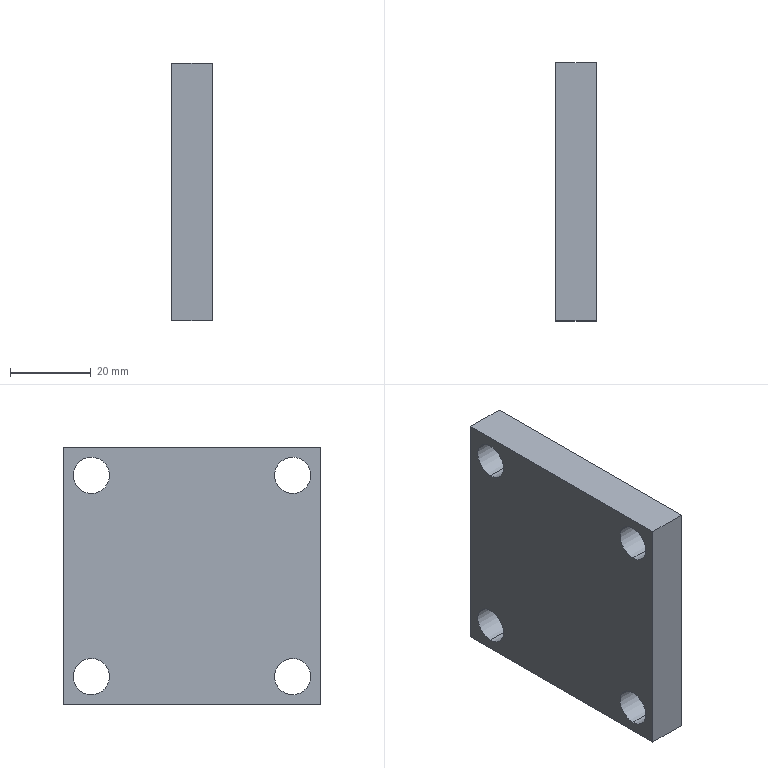Part | STEP file | Positioning_id2310_x_t | 1 solid | 14 faces | box 10 x 64 x 64 mm | volume 38415 mm3 | cylinder 8 | plane 6 | commonest cylinder face diameters 9 x8
STEP:
#1=CARTESIAN_POINT('',(0.,0.,0.));
#2=DIRECTION('',(0.,0.,1.));
#3=DIRECTION('',(1.,0.,0.));
#4=AXIS2_PLACEMENT_3D('',#1,#2,#3);
#5=CARTESIAN_POINT('',(-913.002,325.,173.032));
#6=VERTEX_POINT('',#5);
#7=CARTESIAN_POINT('',(-913.002,325.,164.032));
#8=VERTEX_POINT('',#7);
#9=CARTESIAN_POINT('',(-913.002,325.,168.532));
#10=DIRECTION('',(-1.,0.,0.));
#11=DIRECTION('',(0.,-1.,0.));
#12=AXIS2_PLACEMENT_3D('',#9,#10,#11);
#13=CIRCLE('',#12,4.5);
#14=CARTESIAN_POINT('',(-923.002,325.,168.532));
#15=DIRECTION('',(-1.,0.,0.));
#16=DIRECTION('',(0.,0.,1.));
#17=AXIS2_PLACEMENT_3D('',#14,#15,#16);
#18=CYLINDRICAL_SURFACE('',#17,4.5);
#19=CARTESIAN_POINT('',(-1.571,-10.));
#20=DIRECTION('',(1.,0.));
#21=VECTOR('',#20,1.);
#22=LINE('',#19,#21);
#23=(GEOMETRIC_REPRESENTATION_CONTEXT(2)PARAMETRIC_REPRESENTATION_CONTEXT()REPRESENTATION_CONTEXT('',''));
#24=DEFINITIONAL_REPRESENTATION('',(#22),#23);
#25=PCURVE('',#18,#24);
#26=CARTESIAN_POINT('',(-913.002,284.,218.532));
#27=DIRECTION('',(1.,0.,0.));
#28=DIRECTION('',(0.,1.,0.));
#29=AXIS2_PLACEMENT_3D('',#26,#27,#28);
#30=PLANE('',#29);
#31=CARTESIAN_POINT('',(36.5,-50.));
#32=CARTESIAN_POINT('',(36.5,-42.206));
#33=CARTESIAN_POINT('',(43.25,-46.103));
#34=CARTESIAN_POINT('',(50.,-50.));
#35=CARTESIAN_POINT('',(43.25,-53.897));
#36=CARTESIAN_POINT('',(36.5,-57.794));
#37=CARTESIAN_POINT('',(36.5,-50.));
#38=(BOUNDED_CURVE()B_SPLINE_CURVE(2,(#31,#32,#33,#34,#35,#36,#37),.UNSPECIFIED.,.T.,.F.)B_SPLINE_CURVE_WITH_KNOTS((1,2,2,2,2,1),(-2.094,0.,2.094,4.189,6.283,8.378),.UNSPECIFIED.)CURVE()GEOMETRIC_REPRESENTATION_ITEM()RATIONAL_B_SPLINE_CURVE((1.,0.5,1.,0.5,1.,0.5,1.))REPRESENTATION_ITEM(''));
#39=(GEOMETRIC_REPRESENTATION_CONTEXT(2)PARAMETRIC_REPRESENTATION_CONTEXT()REPRESENTATION_CONTEXT('',''));
#40=DEFINITIONAL_REPRESENTATION('',(#38),#39);
#41=PCURVE('',#30,#40);
#42=SURFACE_CURVE('',#13,(#25,#41),.PCURVE_S1.);
#43=EDGE_CURVE('',#6,#8,#42,.T.);
#44=ORIENTED_EDGE('',*,*,#43,.T.);
#45=CARTESIAN_POINT('',(-923.002,325.,164.032));
#46=VERTEX_POINT('',#45);
#47=CARTESIAN_POINT('',(-923.002,325.,164.032));
#48=DIRECTION('',(1.,0.,0.));
#49=VECTOR('',#48,1.);
#50=LINE('',#47,#49);
#51=CARTESIAN_POINT('',(3.142,0.));
#52=DIRECTION('',(0.,-1.));
#53=VECTOR('',#52,1.);
#54=LINE('',#51,#53);
#55=(GEOMETRIC_REPRESENTATION_CONTEXT(2)PARAMETRIC_REPRESENTATION_CONTEXT()REPRESENTATION_CONTEXT('',''));
#56=DEFINITIONAL_REPRESENTATION('',(#54),#55);
#57=PCURVE('',#18,#56);
#58=CARTESIAN_POINT('',(-923.002,325.,168.532));
#59=DIRECTION('',(-1.,0.,0.));
#60=DIRECTION('',(0.,0.,1.));
#61=AXIS2_PLACEMENT_3D('',#58,#59,#60);
#62=CYLINDRICAL_SURFACE('',#61,4.5);
#63=CARTESIAN_POINT('',(3.142,0.));
#64=DIRECTION('',(0.,-1.));
#65=VECTOR('',#64,1.);
#66=LINE('',#63,#65);
#67=(GEOMETRIC_REPRESENTATION_CONTEXT(2)PARAMETRIC_REPRESENTATION_CONTEXT()REPRESENTATION_CONTEXT('',''));
#68=DEFINITIONAL_REPRESENTATION('',(#66),#67);
#69=PCURVE('',#62,#68);
#70=SURFACE_CURVE('',#50,(#57,#69),.PCURVE_S1.);
#71=EDGE_CURVE('',#46,#8,#70,.T.);
#72=ORIENTED_EDGE('',*,*,#71,.F.);
#73=CARTESIAN_POINT('',(-923.002,325.,173.032));
#74=VERTEX_POINT('',#73);
#75=CARTESIAN_POINT('',(-923.002,325.,168.532));
#76=DIRECTION('',(-1.,0.,0.));
#77=DIRECTION('',(0.,-1.,0.));
#78=AXIS2_PLACEMENT_3D('',#75,#76,#77);
#79=CIRCLE('',#78,4.5);
#80=CARTESIAN_POINT('',(-1.571,0.));
#81=DIRECTION('',(1.,0.));
#82=VECTOR('',#81,1.);
#83=LINE('',#80,#82);
#84=(GEOMETRIC_REPRESENTATION_CONTEXT(2)PARAMETRIC_REPRESENTATION_CONTEXT()REPRESENTATION_CONTEXT('',''));
#85=DEFINITIONAL_REPRESENTATION('',(#83),#84);
#86=PCURVE('',#18,#85);
#87=CARTESIAN_POINT('',(-923.002,284.,218.532));
#88=DIRECTION('',(-1.,0.,0.));
#89=DIRECTION('',(0.,-1.,0.));
#90=AXIS2_PLACEMENT_3D('',#87,#88,#89);
#91=PLANE('',#90);
#92=CARTESIAN_POINT('',(-41.,-50.));
#93=DIRECTION('',(1.,0.));
#94=AXIS2_PLACEMENT_2D('',#92,#93);
#95=CIRCLE('',#94,4.5);
#96=(GEOMETRIC_REPRESENTATION_CONTEXT(2)PARAMETRIC_REPRESENTATION_CONTEXT()REPRESENTATION_CONTEXT('',''));
#97=DEFINITIONAL_REPRESENTATION('',(#95),#96);
#98=PCURVE('',#91,#97);
#99=SURFACE_CURVE('',#79,(#86,#98),.PCURVE_S1.);
#100=EDGE_CURVE('',#74,#46,#99,.T.);
#101=ORIENTED_EDGE('',*,*,#100,.F.);
#102=CARTESIAN_POINT('',(-923.002,325.,173.032));
#103=DIRECTION('',(-1.,0.,0.));
#104=VECTOR('',#103,1.);
#105=LINE('',#102,#104);
#106=CARTESIAN_POINT('',(0.,0.));
#107=DIRECTION('',(0.,1.));
#108=VECTOR('',#107,1.);
#109=LINE('',#106,#108);
#110=(GEOMETRIC_REPRESENTATION_CONTEXT(2)PARAMETRIC_REPRESENTATION_CONTEXT()REPRESENTATION_CONTEXT('',''));
#111=DEFINITIONAL_REPRESENTATION('',(#109),#110);
#112=PCURVE('',#18,#111);
#113=CARTESIAN_POINT('',(6.283,0.));
#114=DIRECTION('',(0.,1.));
#115=VECTOR('',#114,1.);
#116=LINE('',#113,#115);
#117=(GEOMETRIC_REPRESENTATION_CONTEXT(2)PARAMETRIC_REPRESENTATION_CONTEXT()REPRESENTATION_CONTEXT('',''));
#118=DEFINITIONAL_REPRESENTATION('',(#116),#117);
#119=PCURVE('',#62,#118);
#120=SURFACE_CURVE('',#105,(#112,#119),.PCURVE_S1.);
#121=EDGE_CURVE('',#6,#74,#120,.T.);
#122=ORIENTED_EDGE('',*,*,#121,.F.);
#123=EDGE_LOOP('',(#44,#72,#101,#122));
#124=FACE_BOUND('',#123,.F.);
#125=ADVANCED_FACE('',(#124),#18,.F.);
#126=CARTESIAN_POINT('',(-913.002,275.,173.032));
#127=VERTEX_POINT('',#126);
#128=CARTESIAN_POINT('',(-913.002,275.,164.032));
#129=VERTEX_POINT('',#128);
#130=CARTESIAN_POINT('',(-913.002,275.,168.532));
#131=DIRECTION('',(-1.,0.,0.));
#132=DIRECTION('',(0.,-1.,0.));
#133=AXIS2_PLACEMENT_3D('',#130,#131,#132);
#134=CIRCLE('',#133,4.5);
#135=CARTESIAN_POINT('',(-923.002,275.,168.532));
#136=DIRECTION('',(-1.,0.,0.));
#137=DIRECTION('',(0.,0.,1.));
#138=AXIS2_PLACEMENT_3D('',#135,#136,#137);
#139=CYLINDRICAL_SURFACE('',#138,4.5);
#140=CARTESIAN_POINT('',(-1.571,-10.));
#141=DIRECTION('',(1.,0.));
#142=VECTOR('',#141,1.);
#143=LINE('',#140,#142);
#144=(GEOMETRIC_REPRESENTATION_CONTEXT(2)PARAMETRIC_REPRESENTATION_CONTEXT()REPRESENTATION_CONTEXT('',''));
#145=DEFINITIONAL_REPRESENTATION('',(#143),#144);
#146=PCURVE('',#139,#145);
#147=CARTESIAN_POINT('',(-13.5,-50.));
#148=CARTESIAN_POINT('',(-13.5,-42.206));
#149=CARTESIAN_POINT('',(-6.75,-46.103));
#150=CARTESIAN_POINT('',(0.,-50.));
#151=CARTESIAN_POINT('',(-6.75,-53.897));
#152=CARTESIAN_POINT('',(-13.5,-57.794));
#153=CARTESIAN_POINT('',(-13.5,-50.));
#154=(BOUNDED_CURVE()B_SPLINE_CURVE(2,(#147,#148,#149,#150,#151,#152,#153),.UNSPECIFIED.,.T.,.F.)B_SPLINE_CURVE_WITH_KNOTS((1,2,2,2,2,1),(-2.094,0.,2.094,4.189,6.283,8.378),.UNSPECIFIED.)CURVE()GEOMETRIC_REPRESENTATION_ITEM()RATIONAL_B_SPLINE_CURVE((1.,0.5,1.,0.5,1.,0.5,1.))REPRESENTATION_ITEM(''));
#155=(GEOMETRIC_REPRESENTATION_CONTEXT(2)PARAMETRIC_REPRESENTATION_CONTEXT()REPRESENTATION_CONTEXT('',''));
#156=DEFINITIONAL_REPRESENTATION('',(#154),#155);
#157=PCURVE('',#30,#156);
#158=SURFACE_CURVE('',#134,(#146,#157),.PCURVE_S1.);
#159=EDGE_CURVE('',#127,#129,#158,.T.);
#160=ORIENTED_EDGE('',*,*,#159,.T.);
#161=CARTESIAN_POINT('',(-923.002,275.,164.032));
#162=VERTEX_POINT('',#161);
#163=CARTESIAN_POINT('',(-923.002,275.,164.032));
#164=DIRECTION('',(1.,0.,0.));
#165=VECTOR('',#164,1.);
#166=LINE('',#163,#165);
#167=CARTESIAN_POINT('',(3.142,0.));
#168=DIRECTION('',(0.,-1.));
#169=VECTOR('',#168,1.);
#170=LINE('',#167,#169);
#171=(GEOMETRIC_REPRESENTATION_CONTEXT(2)PARAMETRIC_REPRESENTATION_CONTEXT()REPRESENTATION_CONTEXT('',''));
#172=DEFINITIONAL_REPRESENTATION('',(#170),#171);
#173=PCURVE('',#139,#172);
#174=CARTESIAN_POINT('',(-923.002,275.,168.532));
#175=DIRECTION('',(-1.,0.,0.));
#176=DIRECTION('',(0.,0.,1.));
#177=AXIS2_PLACEMENT_3D('',#174,#175,#176);
#178=CYLINDRICAL_SURFACE('',#177,4.5);
#179=CARTESIAN_POINT('',(3.142,0.));
#180=DIRECTION('',(0.,-1.));
#181=VECTOR('',#180,1.);
#182=LINE('',#179,#181);
#183=(GEOMETRIC_REPRESENTATION_CONTEXT(2)PARAMETRIC_REPRESENTATION_CONTEXT()REPRESENTATION_CONTEXT('',''));
#184=DEFINITIONAL_REPRESENTATION('',(#182),#183);
#185=PCURVE('',#178,#184);
#186=SURFACE_CURVE('',#166,(#173,#185),.PCURVE_S1.);
#187=EDGE_CURVE('',#162,#129,#186,.T.);
#188=ORIENTED_EDGE('',*,*,#187,.F.);
#189=CARTESIAN_POINT('',(-923.002,275.,173.032));
#190=VERTEX_POINT('',#189);
#191=CARTESIAN_POINT('',(-923.002,275.,168.532));
#192=DIRECTION('',(-1.,0.,0.));
#193=DIRECTION('',(0.,-1.,0.));
#194=AXIS2_PLACEMENT_3D('',#191,#192,#193);
#195=CIRCLE('',#194,4.5);
#196=CARTESIAN_POINT('',(-1.571,0.));
#197=DIRECTION('',(1.,0.));
#198=VECTOR('',#197,1.);
#199=LINE('',#196,#198);
#200=(GEOMETRIC_REPRESENTATION_CONTEXT(2)PARAMETRIC_REPRESENTATION_CONTEXT()REPRESENTATION_CONTEXT('',''));
#201=DEFINITIONAL_REPRESENTATION('',(#199),#200);
#202=PCURVE('',#139,#201);
#203=CARTESIAN_POINT('',(9.,-50.));
#204=DIRECTION('',(1.,0.));
#205=AXIS2_PLACEMENT_2D('',#203,#204);
#206=CIRCLE('',#205,4.5);
#207=(GEOMETRIC_REPRESENTATION_CONTEXT(2)PARAMETRIC_REPRESENTATION_CONTEXT()REPRESENTATION_CONTEXT('',''));
#208=DEFINITIONAL_REPRESENTATION('',(#206),#207);
#209=PCURVE('',#91,#208);
#210=SURFACE_CURVE('',#195,(#202,#209),.PCURVE_S1.);
#211=EDGE_CURVE('',#190,#162,#210,.T.);
#212=ORIENTED_EDGE('',*,*,#211,.F.);
#213=CARTESIAN_POINT('',(-923.002,275.,173.032));
#214=DIRECTION('',(-1.,0.,0.));
#215=VECTOR('',#214,1.);
#216=LINE('',#213,#215);
#217=CARTESIAN_POINT('',(0.,0.));
#218=DIRECTION('',(0.,1.));
#219=VECTOR('',#218,1.);
#220=LINE('',#217,#219);
#221=(GEOMETRIC_REPRESENTATION_CONTEXT(2)PARAMETRIC_REPRESENTATION_CONTEXT()REPRESENTATION_CONTEXT('',''));
#222=DEFINITIONAL_REPRESENTATION('',(#220),#221);
#223=PCURVE('',#139,#222);
#224=CARTESIAN_POINT('',(6.283,0.));
#225=DIRECTION('',(0.,1.));
#226=VECTOR('',#225,1.);
#227=LINE('',#224,#226);
#228=(GEOMETRIC_REPRESENTATION_CONTEXT(2)PARAMETRIC_REPRESENTATION_CONTEXT()REPRESENTATION_CONTEXT('',''));
#229=DEFINITIONAL_REPRESENTATION('',(#227),#228);
#230=PCURVE('',#178,#229);
#231=SURFACE_CURVE('',#216,(#223,#230),.PCURVE_S1.);
#232=EDGE_CURVE('',#127,#190,#231,.T.);
#233=ORIENTED_EDGE('',*,*,#232,.F.);
#234=EDGE_LOOP('',(#160,#188,#212,#233));
#235=FACE_BOUND('',#234,.F.);
#236=ADVANCED_FACE('',(#235),#139,.F.);
#237=CARTESIAN_POINT('',(-913.002,275.,223.032));
#238=VERTEX_POINT('',#237);
#239=CARTESIAN_POINT('',(-913.002,275.,214.032));
#240=VERTEX_POINT('',#239);
#241=CARTESIAN_POINT('',(-913.002,275.,218.532));
#242=DIRECTION('',(-1.,0.,0.));
#243=DIRECTION('',(0.,-1.,0.));
#244=AXIS2_PLACEMENT_3D('',#241,#242,#243);
#245=CIRCLE('',#244,4.5);
#246=CARTESIAN_POINT('',(-923.002,275.,218.532));
#247=DIRECTION('',(-1.,0.,0.));
#248=DIRECTION('',(0.,0.,1.));
#249=AXIS2_PLACEMENT_3D('',#246,#247,#248);
#250=CYLINDRICAL_SURFACE('',#249,4.5);
#251=CARTESIAN_POINT('',(-1.571,-10.));
#252=DIRECTION('',(1.,0.));
#253=VECTOR('',#252,1.);
#254=LINE('',#251,#253);
#255=(GEOMETRIC_REPRESENTATION_CONTEXT(2)PARAMETRIC_REPRESENTATION_CONTEXT()REPRESENTATION_CONTEXT('',''));
#256=DEFINITIONAL_REPRESENTATION('',(#254),#255);
#257=PCURVE('',#250,#256);
#258=CARTESIAN_POINT('',(-13.5,0.));
#259=CARTESIAN_POINT('',(-13.5,7.794));
#260=CARTESIAN_POINT('',(-6.75,3.897));
#261=CARTESIAN_POINT('',(0.,0.));
#262=CARTESIAN_POINT('',(-6.75,-3.897));
#263=CARTESIAN_POINT('',(-13.5,-7.794));
#264=CARTESIAN_POINT('',(-13.5,0.));
#265=(BOUNDED_CURVE()B_SPLINE_CURVE(2,(#258,#259,#260,#261,#262,#263,#264),.UNSPECIFIED.,.T.,.F.)B_SPLINE_CURVE_WITH_KNOTS((1,2,2,2,2,1),(-2.094,0.,2.094,4.189,6.283,8.378),.UNSPECIFIED.)CURVE()GEOMETRIC_REPRESENTATION_ITEM()RATIONAL_B_SPLINE_CURVE((1.,0.5,1.,0.5,1.,0.5,1.))REPRESENTATION_ITEM(''));
#266=(GEOMETRIC_REPRESENTATION_CONTEXT(2)PARAMETRIC_REPRESENTATION_CONTEXT()REPRESENTATION_CONTEXT('',''));
#267=DEFINITIONAL_REPRESENTATION('',(#265),#266);
#268=PCURVE('',#30,#267);
#269=SURFACE_CURVE('',#245,(#257,#268),.PCURVE_S1.);
#270=EDGE_CURVE('',#238,#240,#269,.T.);
#271=ORIENTED_EDGE('',*,*,#270,.T.);
#272=CARTESIAN_POINT('',(-923.002,275.,214.032));
#273=VERTEX_POINT('',#272);
#274=CARTESIAN_POINT('',(-923.002,275.,214.032));
#275=DIRECTION('',(1.,0.,0.));
#276=VECTOR('',#275,1.);
#277=LINE('',#274,#276);
#278=CARTESIAN_POINT('',(3.142,0.));
#279=DIRECTION('',(0.,-1.));
#280=VECTOR('',#279,1.);
#281=LINE('',#278,#280);
#282=(GEOMETRIC_REPRESENTATION_CONTEXT(2)PARAMETRIC_REPRESENTATION_CONTEXT()REPRESENTATION_CONTEXT('',''));
#283=DEFINITIONAL_REPRESENTATION('',(#281),#282);
#284=PCURVE('',#250,#283);
#285=CARTESIAN_POINT('',(-923.002,275.,218.532));
#286=DIRECTION('',(-1.,0.,0.));
#287=DIRECTION('',(0.,0.,1.));
#288=AXIS2_PLACEMENT_3D('',#285,#286,#287);
#289=CYLINDRICAL_SURFACE('',#288,4.5);
#290=CARTESIAN_POINT('',(3.142,0.));
#291=DIRECTION('',(0.,-1.));
#292=VECTOR('',#291,1.);
#293=LINE('',#290,#292);
#294=(GEOMETRIC_REPRESENTATION_CONTEXT(2)PARAMETRIC_REPRESENTATION_CONTEXT()REPRESENTATION_CONTEXT('',''));
#295=DEFINITIONAL_REPRESENTATION('',(#293),#294);
#296=PCURVE('',#289,#295);
#297=SURFACE_CURVE('',#277,(#284,#296),.PCURVE_S1.);
#298=EDGE_CURVE('',#273,#240,#297,.T.);
#299=ORIENTED_EDGE('',*,*,#298,.F.);
#300=CARTESIAN_POINT('',(-923.002,275.,223.032));
#301=VERTEX_POINT('',#300);
#302=CARTESIAN_POINT('',(-923.002,275.,218.532));
#303=DIRECTION('',(-1.,0.,0.));
#304=DIRECTION('',(0.,-1.,0.));
#305=AXIS2_PLACEMENT_3D('',#302,#303,#304);
#306=CIRCLE('',#305,4.5);
#307=CARTESIAN_POINT('',(-1.571,0.));
#308=DIRECTION('',(1.,0.));
#309=VECTOR('',#308,1.);
#310=LINE('',#307,#309);
#311=(GEOMETRIC_REPRESENTATION_CONTEXT(2)PARAMETRIC_REPRESENTATION_CONTEXT()REPRESENTATION_CONTEXT('',''));
#312=DEFINITIONAL_REPRESENTATION('',(#310),#311);
#313=PCURVE('',#250,#312);
#314=CARTESIAN_POINT('',(9.,0.));
#315=DIRECTION('',(1.,0.));
#316=AXIS2_PLACEMENT_2D('',#314,#315);
#317=CIRCLE('',#316,4.5);
#318=(GEOMETRIC_REPRESENTATION_CONTEXT(2)PARAMETRIC_REPRESENTATION_CONTEXT()REPRESENTATION_CONTEXT('',''));
#319=DEFINITIONAL_REPRESENTATION('',(#317),#318);
#320=PCURVE('',#91,#319);
#321=SURFACE_CURVE('',#306,(#313,#320),.PCURVE_S1.);
#322=EDGE_CURVE('',#301,#273,#321,.T.);
#323=ORIENTED_EDGE('',*,*,#322,.F.);
#324=CARTESIAN_POINT('',(-923.002,275.,223.032));
#325=DIRECTION('',(-1.,0.,0.));
#326=VECTOR('',#325,1.);
#327=LINE('',#324,#326);
#328=CARTESIAN_POINT('',(0.,0.));
#329=DIRECTION('',(0.,1.));
#330=VECTOR('',#329,1.);
#331=LINE('',#328,#330);
#332=(GEOMETRIC_REPRESENTATION_CONTEXT(2)PARAMETRIC_REPRESENTATION_CONTEXT()REPRESENTATION_CONTEXT('',''));
#333=DEFINITIONAL_REPRESENTATION('',(#331),#332);
#334=PCURVE('',#250,#333);
#335=CARTESIAN_POINT('',(6.283,0.));
#336=DIRECTION('',(0.,1.));
#337=VECTOR('',#336,1.);
#338=LINE('',#335,#337);
#339=(GEOMETRIC_REPRESENTATION_CONTEXT(2)PARAMETRIC_REPRESENTATION_CONTEXT()REPRESENTATION_CONTEXT('',''));
#340=DEFINITIONAL_REPRESENTATION('',(#338),#339);
#341=PCURVE('',#289,#340);
#342=SURFACE_CURVE('',#327,(#334,#341),.PCURVE_S1.);
#343=EDGE_CURVE('',#238,#301,#342,.T.);
#344=ORIENTED_EDGE('',*,*,#343,.F.);
#345=EDGE_LOOP('',(#271,#299,#323,#344));
#346=FACE_BOUND('',#345,.F.);
#347=ADVANCED_FACE('',(#346),#250,.F.);
#348=CARTESIAN_POINT('',(-913.002,325.,223.032));
#349=VERTEX_POINT('',#348);
#350=CARTESIAN_POINT('',(-913.002,325.,214.032));
#351=VERTEX_POINT('',#350);
#352=CARTESIAN_POINT('',(-913.002,325.,218.532));
#353=DIRECTION('',(-1.,0.,0.));
#354=DIRECTION('',(0.,-1.,0.));
#355=AXIS2_PLACEMENT_3D('',#352,#353,#354);
#356=CIRCLE('',#355,4.5);
#357=CARTESIAN_POINT('',(-923.002,325.,218.532));
#358=DIRECTION('',(-1.,0.,0.));
#359=DIRECTION('',(0.,0.,1.));
#360=AXIS2_PLACEMENT_3D('',#357,#358,#359);
#361=CYLINDRICAL_SURFACE('',#360,4.5);
#362=CARTESIAN_POINT('',(-1.571,-10.));
#363=DIRECTION('',(1.,0.));
#364=VECTOR('',#363,1.);
#365=LINE('',#362,#364);
#366=(GEOMETRIC_REPRESENTATION_CONTEXT(2)PARAMETRIC_REPRESENTATION_CONTEXT()REPRESENTATION_CONTEXT('',''));
#367=DEFINITIONAL_REPRESENTATION('',(#365),#366);
#368=PCURVE('',#361,#367);
#369=CARTESIAN_POINT('',(36.5,0.));
#370=CARTESIAN_POINT('',(36.5,7.794));
#371=CARTESIAN_POINT('',(43.25,3.897));
#372=CARTESIAN_POINT('',(50.,0.));
#373=CARTESIAN_POINT('',(43.25,-3.897));
#374=CARTESIAN_POINT('',(36.5,-7.794));
#375=CARTESIAN_POINT('',(36.5,0.));
#376=(BOUNDED_CURVE()B_SPLINE_CURVE(2,(#369,#370,#371,#372,#373,#374,#375),.UNSPECIFIED.,.T.,.F.)B_SPLINE_CURVE_WITH_KNOTS((1,2,2,2,2,1),(-2.094,0.,2.094,4.189,6.283,8.378),.UNSPECIFIED.)CURVE()GEOMETRIC_REPRESENTATION_ITEM()RATIONAL_B_SPLINE_CURVE((1.,0.5,1.,0.5,1.,0.5,1.))REPRESENTATION_ITEM(''));
#377=(GEOMETRIC_REPRESENTATION_CONTEXT(2)PARAMETRIC_REPRESENTATION_CONTEXT()REPRESENTATION_CONTEXT('',''));
#378=DEFINITIONAL_REPRESENTATION('',(#376),#377);
#379=PCURVE('',#30,#378);
#380=SURFACE_CURVE('',#356,(#368,#379),.PCURVE_S1.);
#381=EDGE_CURVE('',#349,#351,#380,.T.);
#382=ORIENTED_EDGE('',*,*,#381,.T.);
#383=CARTESIAN_POINT('',(-923.002,325.,214.032));
#384=VERTEX_POINT('',#383);
#385=CARTESIAN_POINT('',(-923.002,325.,214.032));
#386=DIRECTION('',(-1.,0.,0.));
#387=VECTOR('',#386,1.);
#388=LINE('',#385,#387);
#389=CARTESIAN_POINT('',(3.142,0.));
#390=DIRECTION('',(0.,1.));
#391=VECTOR('',#390,1.);
#392=LINE('',#389,#391);
#393=(GEOMETRIC_REPRESENTATION_CONTEXT(2)PARAMETRIC_REPRESENTATION_CONTEXT()REPRESENTATION_CONTEXT('',''));
#394=DEFINITIONAL_REPRESENTATION('',(#392),#393);
#395=PCURVE('',#361,#394);
#396=CARTESIAN_POINT('',(-923.002,325.,218.532));
#397=DIRECTION('',(-1.,0.,0.));
#398=DIRECTION('',(0.,0.,1.));
#399=AXIS2_PLACEMENT_3D('',#396,#397,#398);
#400=CYLINDRICAL_SURFACE('',#399,4.5);
#401=CARTESIAN_POINT('',(3.142,0.));
#402=DIRECTION('',(0.,1.));
#403=VECTOR('',#402,1.);
#404=LINE('',#401,#403);
#405=(GEOMETRIC_REPRESENTATION_CONTEXT(2)PARAMETRIC_REPRESENTATION_CONTEXT()REPRESENTATION_CONTEXT('',''));
#406=DEFINITIONAL_REPRESENTATION('',(#404),#405);
#407=PCURVE('',#400,#406);
#408=SURFACE_CURVE('',#388,(#395,#407),.PCURVE_S1.);
#409=EDGE_CURVE('',#351,#384,#408,.T.);
#410=ORIENTED_EDGE('',*,*,#409,.T.);
#411=CARTESIAN_POINT('',(-923.002,325.,223.032));
#412=VERTEX_POINT('',#411);
#413=CARTESIAN_POINT('',(-923.002,325.,218.532));
#414=DIRECTION('',(-1.,0.,0.));
#415=DIRECTION('',(0.,-1.,0.));
#416=AXIS2_PLACEMENT_3D('',#413,#414,#415);
#417=CIRCLE('',#416,4.5);
#418=CARTESIAN_POINT('',(-1.571,0.));
#419=DIRECTION('',(1.,0.));
#420=VECTOR('',#419,1.);
#421=LINE('',#418,#420);
#422=(GEOMETRIC_REPRESENTATION_CONTEXT(2)PARAMETRIC_REPRESENTATION_CONTEXT()REPRESENTATION_CONTEXT('',''));
#423=DEFINITIONAL_REPRESENTATION('',(#421),#422);
#424=PCURVE('',#361,#423);
#425=CARTESIAN_POINT('',(-41.,0.));
#426=DIRECTION('',(1.,0.));
#427=AXIS2_PLACEMENT_2D('',#425,#426);
#428=CIRCLE('',#427,4.5);
#429=(GEOMETRIC_REPRESENTATION_CONTEXT(2)PARAMETRIC_REPRESENTATION_CONTEXT()REPRESENTATION_CONTEXT('',''));
#430=DEFINITIONAL_REPRESENTATION('',(#428),#429);
#431=PCURVE('',#91,#430);
#432=SURFACE_CURVE('',#417,(#424,#431),.PCURVE_S1.);
#433=EDGE_CURVE('',#412,#384,#432,.T.);
#434=ORIENTED_EDGE('',*,*,#433,.F.);
#435=CARTESIAN_POINT('',(-923.002,325.,223.032));
#436=DIRECTION('',(1.,0.,0.));
#437=VECTOR('',#436,1.);
#438=LINE('',#435,#437);
#439=CARTESIAN_POINT('',(0.,0.));
#440=DIRECTION('',(0.,-1.));
#441=VECTOR('',#440,1.);
#442=LINE('',#439,#441);
#443=(GEOMETRIC_REPRESENTATION_CONTEXT(2)PARAMETRIC_REPRESENTATION_CONTEXT()REPRESENTATION_CONTEXT('',''));
#444=DEFINITIONAL_REPRESENTATION('',(#442),#443);
#445=PCURVE('',#361,#444);
#446=CARTESIAN_POINT('',(6.283,0.));
#447=DIRECTION('',(0.,-1.));
#448=VECTOR('',#447,1.);
#449=LINE('',#446,#448);
#450=(GEOMETRIC_REPRESENTATION_CONTEXT(2)PARAMETRIC_REPRESENTATION_CONTEXT()REPRESENTATION_CONTEXT('',''));
#451=DEFINITIONAL_REPRESENTATION('',(#449),#450);
#452=PCURVE('',#400,#451);
#453=SURFACE_CURVE('',#438,(#445,#452),.PCURVE_S1.);
#454=EDGE_CURVE('',#412,#349,#453,.T.);
#455=ORIENTED_EDGE('',*,*,#454,.T.);
#456=EDGE_LOOP('',(#382,#410,#434,#455));
#457=FACE_BOUND('',#456,.F.);
#458=ADVANCED_FACE('',(#457),#361,.F.);
#459=CARTESIAN_POINT('',(-923.002,268.,161.532));
#460=VERTEX_POINT('',#459);
#461=CARTESIAN_POINT('',(-923.002,268.,225.532));
#462=VERTEX_POINT('',#461);
#463=CARTESIAN_POINT('',(-923.002,268.,161.532));
#464=DIRECTION('',(0.,0.,1.));
#465=VECTOR('',#464,1.);
#466=LINE('',#463,#465);
#467=CARTESIAN_POINT('',(-923.002,268.,218.532));
#468=DIRECTION('',(0.,-1.,0.));
#469=DIRECTION('',(1.,0.,0.));
#470=AXIS2_PLACEMENT_3D('',#467,#468,#469);
#471=PLANE('',#470);
#472=CARTESIAN_POINT('',(0.,-57.));
#473=DIRECTION('',(0.,1.));
#474=VECTOR('',#473,1.);
#475=LINE('',#472,#474);
#476=(GEOMETRIC_REPRESENTATION_CONTEXT(2)PARAMETRIC_REPRESENTATION_CONTEXT()REPRESENTATION_CONTEXT('',''));
#477=DEFINITIONAL_REPRESENTATION('',(#475),#476);
#478=PCURVE('',#471,#477);
#479=CARTESIAN_POINT('',(16.,-57.));
#480=DIRECTION('',(0.,1.));
#481=VECTOR('',#480,1.);
#482=LINE('',#479,#481);
#483=(GEOMETRIC_REPRESENTATION_CONTEXT(2)PARAMETRIC_REPRESENTATION_CONTEXT()REPRESENTATION_CONTEXT('',''));
#484=DEFINITIONAL_REPRESENTATION('',(#482),#483);
#485=PCURVE('',#91,#484);
#486=SURFACE_CURVE('',#466,(#478,#485),.PCURVE_S1.);
#487=EDGE_CURVE('',#460,#462,#486,.T.);
#488=ORIENTED_EDGE('',*,*,#487,.F.);
#489=CARTESIAN_POINT('',(-913.002,268.,161.532));
#490=VERTEX_POINT('',#489);
#491=CARTESIAN_POINT('',(-923.002,268.,161.532));
#492=DIRECTION('',(1.,0.,0.));
#493=VECTOR('',#492,1.);
#494=LINE('',#491,#493);
#495=CARTESIAN_POINT('',(0.,-57.));
#496=DIRECTION('',(1.,0.));
#497=VECTOR('',#496,1.);
#498=LINE('',#495,#497);
#499=(GEOMETRIC_REPRESENTATION_CONTEXT(2)PARAMETRIC_REPRESENTATION_CONTEXT()REPRESENTATION_CONTEXT('',''));
#500=DEFINITIONAL_REPRESENTATION('',(#498),#499);
#501=PCURVE('',#471,#500);
#502=CARTESIAN_POINT('',(-923.002,284.,161.532));
#503=DIRECTION('',(0.,0.,-1.));
#504=DIRECTION('',(1.,0.,0.));
#505=AXIS2_PLACEMENT_3D('',#502,#503,#504);
#506=PLANE('',#505);
#507=CARTESIAN_POINT('',(0.,16.));
#508=DIRECTION('',(1.,0.));
#509=VECTOR('',#508,1.);
#510=LINE('',#507,#509);
#511=(GEOMETRIC_REPRESENTATION_CONTEXT(2)PARAMETRIC_REPRESENTATION_CONTEXT()REPRESENTATION_CONTEXT('',''));
#512=DEFINITIONAL_REPRESENTATION('',(#510),#511);
#513=PCURVE('',#506,#512);
#514=SURFACE_CURVE('',#494,(#501,#513),.PCURVE_S1.);
#515=EDGE_CURVE('',#460,#490,#514,.T.);
#516=ORIENTED_EDGE('',*,*,#515,.T.);
#517=CARTESIAN_POINT('',(-913.002,268.,225.532));
#518=VERTEX_POINT('',#517);
#519=CARTESIAN_POINT('',(-913.002,268.,225.532));
#520=DIRECTION('',(0.,0.,-1.));
#521=VECTOR('',#520,1.);
#522=LINE('',#519,#521);
#523=CARTESIAN_POINT('',(10.,7.));
#524=DIRECTION('',(0.,-1.));
#525=VECTOR('',#524,1.);
#526=LINE('',#523,#525);
#527=(GEOMETRIC_REPRESENTATION_CONTEXT(2)PARAMETRIC_REPRESENTATION_CONTEXT()REPRESENTATION_CONTEXT('',''));
#528=DEFINITIONAL_REPRESENTATION('',(#526),#527);
#529=PCURVE('',#471,#528);
#530=CARTESIAN_POINT('',(-16.,7.));
#531=DIRECTION('',(0.,-1.));
#532=VECTOR('',#531,1.);
#533=LINE('',#530,#532);
#534=(GEOMETRIC_REPRESENTATION_CONTEXT(2)PARAMETRIC_REPRESENTATION_CONTEXT()REPRESENTATION_CONTEXT('',''));
#535=DEFINITIONAL_REPRESENTATION('',(#533),#534);
#536=PCURVE('',#30,#535);
#537=SURFACE_CURVE('',#522,(#529,#536),.PCURVE_S1.);
#538=EDGE_CURVE('',#518,#490,#537,.T.);
#539=ORIENTED_EDGE('',*,*,#538,.F.);
#540=CARTESIAN_POINT('',(-923.002,268.,225.532));
#541=DIRECTION('',(1.,0.,0.));
#542=VECTOR('',#541,1.);
#543=LINE('',#540,#542);
#544=CARTESIAN_POINT('',(0.,7.));
#545=DIRECTION('',(1.,0.));
#546=VECTOR('',#545,1.);
#547=LINE('',#544,#546);
#548=(GEOMETRIC_REPRESENTATION_CONTEXT(2)PARAMETRIC_REPRESENTATION_CONTEXT()REPRESENTATION_CONTEXT('',''));
#549=DEFINITIONAL_REPRESENTATION('',(#547),#548);
#550=PCURVE('',#471,#549);
#551=CARTESIAN_POINT('',(-923.002,284.,225.532));
#552=DIRECTION('',(0.,0.,1.));
#553=DIRECTION('',(-1.,0.,0.));
#554=AXIS2_PLACEMENT_3D('',#551,#552,#553);
#555=PLANE('',#554);
#556=CARTESIAN_POINT('',(0.,16.));
#557=DIRECTION('',(-1.,0.));
#558=VECTOR('',#557,1.);
#559=LINE('',#556,#558);
#560=(GEOMETRIC_REPRESENTATION_CONTEXT(2)PARAMETRIC_REPRESENTATION_CONTEXT()REPRESENTATION_CONTEXT('',''));
#561=DEFINITIONAL_REPRESENTATION('',(#559),#560);
#562=PCURVE('',#555,#561);
#563=SURFACE_CURVE('',#543,(#550,#562),.PCURVE_S1.);
#564=EDGE_CURVE('',#462,#518,#563,.T.);
#565=ORIENTED_EDGE('',*,*,#564,.F.);
#566=EDGE_LOOP('',(#488,#516,#539,#565));
#567=FACE_BOUND('',#566,.T.);
#568=ADVANCED_FACE('',(#567),#471,.T.);
#569=CARTESIAN_POINT('',(-923.002,325.,214.032));
#570=CARTESIAN_POINT('',(-923.002,320.5,214.032));
#571=CARTESIAN_POINT('',(-923.002,318.25,218.532));
#572=CARTESIAN_POINT('',(-923.002,320.5,223.032));
#573=CARTESIAN_POINT('',(-923.002,325.,223.032));
#574=(BOUNDED_CURVE()B_SPLINE_CURVE(4,(#569,#570,#571,#572,#573),.UNSPECIFIED.,.F.,.F.)B_SPLINE_CURVE_WITH_KNOTS((5,5),(0.,1.),.PIECEWISE_BEZIER_KNOTS.)CURVE()GEOMETRIC_REPRESENTATION_ITEM()RATIONAL_B_SPLINE_CURVE((1.,0.7071,0.6667,0.7071,1.))REPRESENTATION_ITEM(''));
#575=CARTESIAN_POINT('',(-41.,-4.5));
#576=CARTESIAN_POINT('',(-36.5,-4.5));
#577=CARTESIAN_POINT('',(-34.25,0.));
#578=CARTESIAN_POINT('',(-36.5,4.5));
#579=CARTESIAN_POINT('',(-41.,4.5));
#580=(BOUNDED_CURVE()B_SPLINE_CURVE(4,(#575,#576,#577,#578,#579),.UNSPECIFIED.,.F.,.F.)B_SPLINE_CURVE_WITH_KNOTS((5,5),(0.,1.),.PIECEWISE_BEZIER_KNOTS.)CURVE()GEOMETRIC_REPRESENTATION_ITEM()RATIONAL_B_SPLINE_CURVE((1.,0.7071,0.6667,0.7071,1.))REPRESENTATION_ITEM(''));
#581=(GEOMETRIC_REPRESENTATION_CONTEXT(2)PARAMETRIC_REPRESENTATION_CONTEXT()REPRESENTATION_CONTEXT('',''));
#582=DEFINITIONAL_REPRESENTATION('',(#580),#581);
#583=PCURVE('',#91,#582);
#584=CARTESIAN_POINT('',(3.142,0.));
#585=CARTESIAN_POINT('',(3.184,0.));
#586=CARTESIAN_POINT('',(3.271,0.));
#587=CARTESIAN_POINT('',(3.405,0.));
#588=CARTESIAN_POINT('',(3.542,0.));
#589=CARTESIAN_POINT('',(3.681,0.));
#590=CARTESIAN_POINT('',(3.823,0.));
#591=CARTESIAN_POINT('',(3.968,0.));
#592=CARTESIAN_POINT('',(4.114,0.));
#593=CARTESIAN_POINT('',(4.262,0.));
#594=CARTESIAN_POINT('',(4.412,0.));
#595=CARTESIAN_POINT('',(4.562,0.));
#596=CARTESIAN_POINT('',(4.712,0.));
#597=CARTESIAN_POINT('',(4.863,0.));
#598=CARTESIAN_POINT('',(5.013,0.));
#599=CARTESIAN_POINT('',(5.163,0.));
#600=CARTESIAN_POINT('',(5.311,0.));
#601=CARTESIAN_POINT('',(5.457,0.));
#602=CARTESIAN_POINT('',(5.602,0.));
#603=CARTESIAN_POINT('',(5.744,0.));
#604=CARTESIAN_POINT('',(5.883,0.));
#605=CARTESIAN_POINT('',(6.02,0.));
#606=CARTESIAN_POINT('',(6.153,0.));
#607=CARTESIAN_POINT('',(6.24,0.));
#608=CARTESIAN_POINT('',(6.283,0.));
#609=B_SPLINE_CURVE_WITH_KNOTS('',3,(#584,#585,#586,#587,#588,#589,#590,#591,#592,#593,#594,#595,#596,#597,#598,#599,#600,#601,#602,#603,#604,#605,#606,#607,#608),.UNSPECIFIED.,.F.,.F.,(4,1,1,1,1,1,1,1,1,1,1,1,1,1,1,1,1,1,1,1,1,1,4),(0.,0.04545,0.09091,0.1364,0.1818,0.2273,0.2727,0.3182,0.3636,0.4091,0.4545,0.5,0.5455,0.5909,0.6364,0.6818,0.7273,0.7727,0.8182,0.8636,0.9091,0.9545,1.),.QUASI_UNIFORM_KNOTS.);
#610=(GEOMETRIC_REPRESENTATION_CONTEXT(2)PARAMETRIC_REPRESENTATION_CONTEXT()REPRESENTATION_CONTEXT('',''));
#611=DEFINITIONAL_REPRESENTATION('',(#609),#610);
#612=PCURVE('',#400,#611);
#613=SURFACE_CURVE('',#574,(#583,#612),.PCURVE_S1.);
#614=EDGE_CURVE('',#384,#412,#613,.T.);
#615=ORIENTED_EDGE('',*,*,#614,.F.);
#616=ORIENTED_EDGE('',*,*,#433,.F.);
#617=EDGE_LOOP('',(#615,#616));
#618=FACE_BOUND('',#617,.T.);
#619=CARTESIAN_POINT('',(-923.002,275.,214.032));
#620=CARTESIAN_POINT('',(-923.002,270.5,214.032));
#621=CARTESIAN_POINT('',(-923.002,268.25,218.532));
#622=CARTESIAN_POINT('',(-923.002,270.5,223.032));
#623=CARTESIAN_POINT('',(-923.002,275.,223.032));
#624=(BOUNDED_CURVE()B_SPLINE_CURVE(4,(#619,#620,#621,#622,#623),.UNSPECIFIED.,.F.,.F.)B_SPLINE_CURVE_WITH_KNOTS((5,5),(0.,1.),.PIECEWISE_BEZIER_KNOTS.)CURVE()GEOMETRIC_REPRESENTATION_ITEM()RATIONAL_B_SPLINE_CURVE((1.,0.7071,0.6667,0.7071,1.))REPRESENTATION_ITEM(''));
#625=CARTESIAN_POINT('',(9.,-4.5));
#626=CARTESIAN_POINT('',(13.5,-4.5));
#627=CARTESIAN_POINT('',(15.75,0.));
#628=CARTESIAN_POINT('',(13.5,4.5));
#629=CARTESIAN_POINT('',(9.,4.5));
#630=(BOUNDED_CURVE()B_SPLINE_CURVE(4,(#625,#626,#627,#628,#629),.UNSPECIFIED.,.F.,.F.)B_SPLINE_CURVE_WITH_KNOTS((5,5),(0.,1.),.PIECEWISE_BEZIER_KNOTS.)CURVE()GEOMETRIC_REPRESENTATION_ITEM()RATIONAL_B_SPLINE_CURVE((1.,0.7071,0.6667,0.7071,1.))REPRESENTATION_ITEM(''));
#631=(GEOMETRIC_REPRESENTATION_CONTEXT(2)PARAMETRIC_REPRESENTATION_CONTEXT()REPRESENTATION_CONTEXT('',''));
#632=DEFINITIONAL_REPRESENTATION('',(#630),#631);
#633=PCURVE('',#91,#632);
#634=CARTESIAN_POINT('',(3.142,0.));
#635=CARTESIAN_POINT('',(3.184,0.));
#636=CARTESIAN_POINT('',(3.271,0.));
#637=CARTESIAN_POINT('',(3.405,0.));
#638=CARTESIAN_POINT('',(3.542,0.));
#639=CARTESIAN_POINT('',(3.681,0.));
#640=CARTESIAN_POINT('',(3.823,0.));
#641=CARTESIAN_POINT('',(3.968,0.));
#642=CARTESIAN_POINT('',(4.114,0.));
#643=CARTESIAN_POINT('',(4.262,0.));
#644=CARTESIAN_POINT('',(4.412,0.));
#645=CARTESIAN_POINT('',(4.562,0.));
#646=CARTESIAN_POINT('',(4.712,0.));
#647=CARTESIAN_POINT('',(4.863,0.));
#648=CARTESIAN_POINT('',(5.013,0.));
#649=CARTESIAN_POINT('',(5.163,0.));
#650=CARTESIAN_POINT('',(5.311,0.));
#651=CARTESIAN_POINT('',(5.457,0.));
#652=CARTESIAN_POINT('',(5.602,0.));
#653=CARTESIAN_POINT('',(5.744,0.));
#654=CARTESIAN_POINT('',(5.883,0.));
#655=CARTESIAN_POINT('',(6.02,0.));
#656=CARTESIAN_POINT('',(6.153,0.));
#657=CARTESIAN_POINT('',(6.24,0.));
#658=CARTESIAN_POINT('',(6.283,0.));
#659=B_SPLINE_CURVE_WITH_KNOTS('',3,(#634,#635,#636,#637,#638,#639,#640,#641,#642,#643,#644,#645,#646,#647,#648,#649,#650,#651,#652,#653,#654,#655,#656,#657,#658),.UNSPECIFIED.,.F.,.F.,(4,1,1,1,1,1,1,1,1,1,1,1,1,1,1,1,1,1,1,1,1,1,4),(0.,0.04545,0.09091,0.1364,0.1818,0.2273,0.2727,0.3182,0.3636,0.4091,0.4545,0.5,0.5455,0.5909,0.6364,0.6818,0.7273,0.7727,0.8182,0.8636,0.9091,0.9545,1.),.QUASI_UNIFORM_KNOTS.);
#660=(GEOMETRIC_REPRESENTATION_CONTEXT(2)PARAMETRIC_REPRESENTATION_CONTEXT()REPRESENTATION_CONTEXT('',''));
#661=DEFINITIONAL_REPRESENTATION('',(#659),#660);
#662=PCURVE('',#289,#661);
#663=SURFACE_CURVE('',#624,(#633,#662),.PCURVE_S1.);
#664=EDGE_CURVE('',#273,#301,#663,.T.);
#665=ORIENTED_EDGE('',*,*,#664,.F.);
#666=ORIENTED_EDGE('',*,*,#322,.F.);
#667=EDGE_LOOP('',(#665,#666));
#668=FACE_BOUND('',#667,.T.);
#669=CARTESIAN_POINT('',(-923.002,275.,164.032));
#670=CARTESIAN_POINT('',(-923.002,270.5,164.032));
#671=CARTESIAN_POINT('',(-923.002,268.25,168.532));
#672=CARTESIAN_POINT('',(-923.002,270.5,173.032));
#673=CARTESIAN_POINT('',(-923.002,275.,173.032));
#674=(BOUNDED_CURVE()B_SPLINE_CURVE(4,(#669,#670,#671,#672,#673),.UNSPECIFIED.,.F.,.F.)B_SPLINE_CURVE_WITH_KNOTS((5,5),(0.,1.),.PIECEWISE_BEZIER_KNOTS.)CURVE()GEOMETRIC_REPRESENTATION_ITEM()RATIONAL_B_SPLINE_CURVE((1.,0.7071,0.6667,0.7071,1.))REPRESENTATION_ITEM(''));
#675=CARTESIAN_POINT('',(9.,-54.5));
#676=CARTESIAN_POINT('',(13.5,-54.5));
#677=CARTESIAN_POINT('',(15.75,-50.));
#678=CARTESIAN_POINT('',(13.5,-45.5));
#679=CARTESIAN_POINT('',(9.,-45.5));
#680=(BOUNDED_CURVE()B_SPLINE_CURVE(4,(#675,#676,#677,#678,#679),.UNSPECIFIED.,.F.,.F.)B_SPLINE_CURVE_WITH_KNOTS((5,5),(0.,1.),.PIECEWISE_BEZIER_KNOTS.)CURVE()GEOMETRIC_REPRESENTATION_ITEM()RATIONAL_B_SPLINE_CURVE((1.,0.7071,0.6667,0.7071,1.))REPRESENTATION_ITEM(''));
#681=(GEOMETRIC_REPRESENTATION_CONTEXT(2)PARAMETRIC_REPRESENTATION_CONTEXT()REPRESENTATION_CONTEXT('',''));
#682=DEFINITIONAL_REPRESENTATION('',(#680),#681);
#683=PCURVE('',#91,#682);
#684=CARTESIAN_POINT('',(3.142,0.));
#685=CARTESIAN_POINT('',(3.184,0.));
#686=CARTESIAN_POINT('',(3.271,0.));
#687=CARTESIAN_POINT('',(3.405,0.));
#688=CARTESIAN_POINT('',(3.542,0.));
#689=CARTESIAN_POINT('',(3.681,0.));
#690=CARTESIAN_POINT('',(3.823,0.));
#691=CARTESIAN_POINT('',(3.968,0.));
#692=CARTESIAN_POINT('',(4.114,0.));
#693=CARTESIAN_POINT('',(4.262,0.));
#694=CARTESIAN_POINT('',(4.412,0.));
#695=CARTESIAN_POINT('',(4.562,0.));
#696=CARTESIAN_POINT('',(4.712,0.));
#697=CARTESIAN_POINT('',(4.863,0.));
#698=CARTESIAN_POINT('',(5.013,0.));
#699=CARTESIAN_POINT('',(5.163,0.));
#700=CARTESIAN_POINT('',(5.311,0.));
#701=CARTESIAN_POINT('',(5.457,0.));
#702=CARTESIAN_POINT('',(5.602,0.));
#703=CARTESIAN_POINT('',(5.744,0.));
#704=CARTESIAN_POINT('',(5.883,0.));
#705=CARTESIAN_POINT('',(6.02,0.));
#706=CARTESIAN_POINT('',(6.153,0.));
#707=CARTESIAN_POINT('',(6.24,0.));
#708=CARTESIAN_POINT('',(6.283,0.));
#709=B_SPLINE_CURVE_WITH_KNOTS('',3,(#684,#685,#686,#687,#688,#689,#690,#691,#692,#693,#694,#695,#696,#697,#698,#699,#700,#701,#702,#703,#704,#705,#706,#707,#708),.UNSPECIFIED.,.F.,.F.,(4,1,1,1,1,1,1,1,1,1,1,1,1,1,1,1,1,1,1,1,1,1,4),(0.,0.04545,0.09091,0.1364,0.1818,0.2273,0.2727,0.3182,0.3636,0.4091,0.4545,0.5,0.5455,0.5909,0.6364,0.6818,0.7273,0.7727,0.8182,0.8636,0.9091,0.9545,1.),.QUASI_UNIFORM_KNOTS.);
#710=(GEOMETRIC_REPRESENTATION_CONTEXT(2)PARAMETRIC_REPRESENTATION_CONTEXT()REPRESENTATION_CONTEXT('',''));
#711=DEFINITIONAL_REPRESENTATION('',(#709),#710);
#712=PCURVE('',#178,#711);
#713=SURFACE_CURVE('',#674,(#683,#712),.PCURVE_S1.);
#714=EDGE_CURVE('',#162,#190,#713,.T.);
#715=ORIENTED_EDGE('',*,*,#714,.F.);
#716=ORIENTED_EDGE('',*,*,#211,.F.);
#717=EDGE_LOOP('',(#715,#716));
#718=FACE_BOUND('',#717,.T.);
#719=CARTESIAN_POINT('',(-923.002,325.,164.032));
#720=CARTESIAN_POINT('',(-923.002,320.5,164.032));
#721=CARTESIAN_POINT('',(-923.002,318.25,168.532));
#722=CARTESIAN_POINT('',(-923.002,320.5,173.032));
#723=CARTESIAN_POINT('',(-923.002,325.,173.032));
#724=(BOUNDED_CURVE()B_SPLINE_CURVE(4,(#719,#720,#721,#722,#723),.UNSPECIFIED.,.F.,.F.)B_SPLINE_CURVE_WITH_KNOTS((5,5),(0.,1.),.PIECEWISE_BEZIER_KNOTS.)CURVE()GEOMETRIC_REPRESENTATION_ITEM()RATIONAL_B_SPLINE_CURVE((1.,0.7071,0.6667,0.7071,1.))REPRESENTATION_ITEM(''));
#725=CARTESIAN_POINT('',(-41.,-54.5));
#726=CARTESIAN_POINT('',(-36.5,-54.5));
#727=CARTESIAN_POINT('',(-34.25,-50.));
#728=CARTESIAN_POINT('',(-36.5,-45.5));
#729=CARTESIAN_POINT('',(-41.,-45.5));
#730=(BOUNDED_CURVE()B_SPLINE_CURVE(4,(#725,#726,#727,#728,#729),.UNSPECIFIED.,.F.,.F.)B_SPLINE_CURVE_WITH_KNOTS((5,5),(0.,1.),.PIECEWISE_BEZIER_KNOTS.)CURVE()GEOMETRIC_REPRESENTATION_ITEM()RATIONAL_B_SPLINE_CURVE((1.,0.7071,0.6667,0.7071,1.))REPRESENTATION_ITEM(''));
#731=(GEOMETRIC_REPRESENTATION_CONTEXT(2)PARAMETRIC_REPRESENTATION_CONTEXT()REPRESENTATION_CONTEXT('',''));
#732=DEFINITIONAL_REPRESENTATION('',(#730),#731);
#733=PCURVE('',#91,#732);
#734=CARTESIAN_POINT('',(3.142,0.));
#735=CARTESIAN_POINT('',(3.184,0.));
#736=CARTESIAN_POINT('',(3.271,0.));
#737=CARTESIAN_POINT('',(3.405,0.));
#738=CARTESIAN_POINT('',(3.542,0.));
#739=CARTESIAN_POINT('',(3.681,0.));
#740=CARTESIAN_POINT('',(3.823,0.));
#741=CARTESIAN_POINT('',(3.968,0.));
#742=CARTESIAN_POINT('',(4.114,0.));
#743=CARTESIAN_POINT('',(4.262,0.));
#744=CARTESIAN_POINT('',(4.412,0.));
#745=CARTESIAN_POINT('',(4.562,0.));
#746=CARTESIAN_POINT('',(4.712,0.));
#747=CARTESIAN_POINT('',(4.863,0.));
#748=CARTESIAN_POINT('',(5.013,0.));
#749=CARTESIAN_POINT('',(5.163,0.));
#750=CARTESIAN_POINT('',(5.311,0.));
#751=CARTESIAN_POINT('',(5.457,0.));
#752=CARTESIAN_POINT('',(5.602,0.));
#753=CARTESIAN_POINT('',(5.744,0.));
#754=CARTESIAN_POINT('',(5.883,0.));
#755=CARTESIAN_POINT('',(6.02,0.));
#756=CARTESIAN_POINT('',(6.153,0.));
#757=CARTESIAN_POINT('',(6.24,0.));
#758=CARTESIAN_POINT('',(6.283,0.));
#759=B_SPLINE_CURVE_WITH_KNOTS('',3,(#734,#735,#736,#737,#738,#739,#740,#741,#742,#743,#744,#745,#746,#747,#748,#749,#750,#751,#752,#753,#754,#755,#756,#757,#758),.UNSPECIFIED.,.F.,.F.,(4,1,1,1,1,1,1,1,1,1,1,1,1,1,1,1,1,1,1,1,1,1,4),(0.,0.04545,0.09091,0.1364,0.1818,0.2273,0.2727,0.3182,0.3636,0.4091,0.4545,0.5,0.5455,0.5909,0.6364,0.6818,0.7273,0.7727,0.8182,0.8636,0.9091,0.9545,1.),.QUASI_UNIFORM_KNOTS.);
#760=(GEOMETRIC_REPRESENTATION_CONTEXT(2)PARAMETRIC_REPRESENTATION_CONTEXT()REPRESENTATION_CONTEXT('',''));
#761=DEFINITIONAL_REPRESENTATION('',(#759),#760);
#762=PCURVE('',#62,#761);
#763=SURFACE_CURVE('',#724,(#733,#762),.PCURVE_S1.);
#764=EDGE_CURVE('',#46,#74,#763,.T.);
#765=ORIENTED_EDGE('',*,*,#764,.F.);
#766=ORIENTED_EDGE('',*,*,#100,.F.);
#767=EDGE_LOOP('',(#765,#766));
#768=FACE_BOUND('',#767,.T.);
#769=ORIENTED_EDGE('',*,*,#487,.T.);
#770=CARTESIAN_POINT('',(-923.002,332.,225.532));
#771=VERTEX_POINT('',#770);
#772=CARTESIAN_POINT('',(-923.002,268.,225.532));
#773=DIRECTION('',(0.,1.,0.));
#774=VECTOR('',#773,1.);
#775=LINE('',#772,#774);
#776=CARTESIAN_POINT('',(16.,7.));
#777=DIRECTION('',(-1.,0.));
#778=VECTOR('',#777,1.);
#779=LINE('',#776,#778);
#780=(GEOMETRIC_REPRESENTATION_CONTEXT(2)PARAMETRIC_REPRESENTATION_CONTEXT()REPRESENTATION_CONTEXT('',''));
#781=DEFINITIONAL_REPRESENTATION('',(#779),#780);
#782=PCURVE('',#91,#781);
#783=CARTESIAN_POINT('',(0.,16.));
#784=DIRECTION('',(0.,-1.));
#785=VECTOR('',#784,1.);
#786=LINE('',#783,#785);
#787=(GEOMETRIC_REPRESENTATION_CONTEXT(2)PARAMETRIC_REPRESENTATION_CONTEXT()REPRESENTATION_CONTEXT('',''));
#788=DEFINITIONAL_REPRESENTATION('',(#786),#787);
#789=PCURVE('',#555,#788);
#790=SURFACE_CURVE('',#775,(#782,#789),.PCURVE_S1.);
#791=EDGE_CURVE('',#462,#771,#790,.T.);
#792=ORIENTED_EDGE('',*,*,#791,.T.);
#793=CARTESIAN_POINT('',(-923.002,332.,161.532));
#794=VERTEX_POINT('',#793);
#795=CARTESIAN_POINT('',(-923.002,332.,225.532));
#796=DIRECTION('',(0.,0.,-1.));
#797=VECTOR('',#796,1.);
#798=LINE('',#795,#797);
#799=CARTESIAN_POINT('',(-48.,7.));
#800=DIRECTION('',(0.,-1.));
#801=VECTOR('',#800,1.);
#802=LINE('',#799,#801);
#803=(GEOMETRIC_REPRESENTATION_CONTEXT(2)PARAMETRIC_REPRESENTATION_CONTEXT()REPRESENTATION_CONTEXT('',''));
#804=DEFINITIONAL_REPRESENTATION('',(#802),#803);
#805=PCURVE('',#91,#804);
#806=CARTESIAN_POINT('',(-923.002,332.,218.532));
#807=DIRECTION('',(0.,1.,0.));
#808=DIRECTION('',(-1.,0.,0.));
#809=AXIS2_PLACEMENT_3D('',#806,#807,#808);
#810=PLANE('',#809);
#811=CARTESIAN_POINT('',(0.,7.));
#812=DIRECTION('',(0.,-1.));
#813=VECTOR('',#812,1.);
#814=LINE('',#811,#813);
#815=(GEOMETRIC_REPRESENTATION_CONTEXT(2)PARAMETRIC_REPRESENTATION_CONTEXT()REPRESENTATION_CONTEXT('',''));
#816=DEFINITIONAL_REPRESENTATION('',(#814),#815);
#817=PCURVE('',#810,#816);
#818=SURFACE_CURVE('',#798,(#805,#817),.PCURVE_S1.);
#819=EDGE_CURVE('',#771,#794,#818,.T.);
#820=ORIENTED_EDGE('',*,*,#819,.T.);
#821=CARTESIAN_POINT('',(-923.002,332.,161.532));
#822=DIRECTION('',(0.,-1.,0.));
#823=VECTOR('',#822,1.);
#824=LINE('',#821,#823);
#825=CARTESIAN_POINT('',(-48.,-57.));
#826=DIRECTION('',(1.,0.));
#827=VECTOR('',#826,1.);
#828=LINE('',#825,#827);
#829=(GEOMETRIC_REPRESENTATION_CONTEXT(2)PARAMETRIC_REPRESENTATION_CONTEXT()REPRESENTATION_CONTEXT('',''));
#830=DEFINITIONAL_REPRESENTATION('',(#828),#829);
#831=PCURVE('',#91,#830);
#832=CARTESIAN_POINT('',(0.,-48.));
#833=DIRECTION('',(0.,1.));
#834=VECTOR('',#833,1.);
#835=LINE('',#832,#834);
#836=(GEOMETRIC_REPRESENTATION_CONTEXT(2)PARAMETRIC_REPRESENTATION_CONTEXT()REPRESENTATION_CONTEXT('',''));
#837=DEFINITIONAL_REPRESENTATION('',(#835),#836);
#838=PCURVE('',#506,#837);
#839=SURFACE_CURVE('',#824,(#831,#838),.PCURVE_S1.);
#840=EDGE_CURVE('',#794,#460,#839,.T.);
#841=ORIENTED_EDGE('',*,*,#840,.T.);
#842=EDGE_LOOP('',(#769,#792,#820,#841));
#843=FACE_BOUND('',#842,.T.);
#844=ADVANCED_FACE('',(#618,#668,#718,#768,#843),#91,.T.);
#845=CARTESIAN_POINT('',(-913.002,332.,225.532));
#846=VERTEX_POINT('',#845);
#847=CARTESIAN_POINT('',(-923.002,332.,225.532));
#848=DIRECTION('',(1.,0.,0.));
#849=VECTOR('',#848,1.);
#850=LINE('',#847,#849);
#851=CARTESIAN_POINT('',(0.,-48.));
#852=DIRECTION('',(-1.,0.));
#853=VECTOR('',#852,1.);
#854=LINE('',#851,#853);
#855=(GEOMETRIC_REPRESENTATION_CONTEXT(2)PARAMETRIC_REPRESENTATION_CONTEXT()REPRESENTATION_CONTEXT('',''));
#856=DEFINITIONAL_REPRESENTATION('',(#854),#855);
#857=PCURVE('',#555,#856);
#858=CARTESIAN_POINT('',(0.,7.));
#859=DIRECTION('',(-1.,0.));
#860=VECTOR('',#859,1.);
#861=LINE('',#858,#860);
#862=(GEOMETRIC_REPRESENTATION_CONTEXT(2)PARAMETRIC_REPRESENTATION_CONTEXT()REPRESENTATION_CONTEXT('',''));
#863=DEFINITIONAL_REPRESENTATION('',(#861),#862);
#864=PCURVE('',#810,#863);
#865=SURFACE_CURVE('',#850,(#857,#864),.PCURVE_S1.);
#866=EDGE_CURVE('',#771,#846,#865,.T.);
#867=ORIENTED_EDGE('',*,*,#866,.F.);
#868=ORIENTED_EDGE('',*,*,#791,.F.);
#869=ORIENTED_EDGE('',*,*,#564,.T.);
#870=CARTESIAN_POINT('',(-913.002,332.,225.532));
#871=DIRECTION('',(0.,-1.,0.));
#872=VECTOR('',#871,1.);
#873=LINE('',#870,#872);
#874=CARTESIAN_POINT('',(-10.,-48.));
#875=DIRECTION('',(0.,1.));
#876=VECTOR('',#875,1.);
#877=LINE('',#874,#876);
#878=(GEOMETRIC_REPRESENTATION_CONTEXT(2)PARAMETRIC_REPRESENTATION_CONTEXT()REPRESENTATION_CONTEXT('',''));
#879=DEFINITIONAL_REPRESENTATION('',(#877),#878);
#880=PCURVE('',#555,#879);
#881=CARTESIAN_POINT('',(48.,7.));
#882=DIRECTION('',(-1.,0.));
#883=VECTOR('',#882,1.);
#884=LINE('',#881,#883);
#885=(GEOMETRIC_REPRESENTATION_CONTEXT(2)PARAMETRIC_REPRESENTATION_CONTEXT()REPRESENTATION_CONTEXT('',''));
#886=DEFINITIONAL_REPRESENTATION('',(#884),#885);
#887=PCURVE('',#30,#886);
#888=SURFACE_CURVE('',#873,(#880,#887),.PCURVE_S1.);
#889=EDGE_CURVE('',#846,#518,#888,.T.);
#890=ORIENTED_EDGE('',*,*,#889,.F.);
#891=EDGE_LOOP('',(#867,#868,#869,#890));
#892=FACE_BOUND('',#891,.T.);
#893=ADVANCED_FACE('',(#892),#555,.T.);
#894=CARTESIAN_POINT('',(-913.002,332.,161.532));
#895=VERTEX_POINT('',#894);
#896=CARTESIAN_POINT('',(-923.002,332.,161.532));
#897=DIRECTION('',(1.,0.,0.));
#898=VECTOR('',#897,1.);
#899=LINE('',#896,#898);
#900=CARTESIAN_POINT('',(0.,-57.));
#901=DIRECTION('',(-1.,0.));
#902=VECTOR('',#901,1.);
#903=LINE('',#900,#902);
#904=(GEOMETRIC_REPRESENTATION_CONTEXT(2)PARAMETRIC_REPRESENTATION_CONTEXT()REPRESENTATION_CONTEXT('',''));
#905=DEFINITIONAL_REPRESENTATION('',(#903),#904);
#906=PCURVE('',#810,#905);
#907=CARTESIAN_POINT('',(0.,-48.));
#908=DIRECTION('',(1.,0.));
#909=VECTOR('',#908,1.);
#910=LINE('',#907,#909);
#911=(GEOMETRIC_REPRESENTATION_CONTEXT(2)PARAMETRIC_REPRESENTATION_CONTEXT()REPRESENTATION_CONTEXT('',''));
#912=DEFINITIONAL_REPRESENTATION('',(#910),#911);
#913=PCURVE('',#506,#912);
#914=SURFACE_CURVE('',#899,(#906,#913),.PCURVE_S1.);
#915=EDGE_CURVE('',#794,#895,#914,.T.);
#916=ORIENTED_EDGE('',*,*,#915,.F.);
#917=ORIENTED_EDGE('',*,*,#819,.F.);
#918=ORIENTED_EDGE('',*,*,#866,.T.);
#919=CARTESIAN_POINT('',(-913.002,332.,161.532));
#920=DIRECTION('',(0.,0.,1.));
#921=VECTOR('',#920,1.);
#922=LINE('',#919,#921);
#923=CARTESIAN_POINT('',(-10.,-57.));
#924=DIRECTION('',(0.,1.));
#925=VECTOR('',#924,1.);
#926=LINE('',#923,#925);
#927=(GEOMETRIC_REPRESENTATION_CONTEXT(2)PARAMETRIC_REPRESENTATION_CONTEXT()REPRESENTATION_CONTEXT('',''));
#928=DEFINITIONAL_REPRESENTATION('',(#926),#927);
#929=PCURVE('',#810,#928);
#930=CARTESIAN_POINT('',(48.,-57.));
#931=DIRECTION('',(0.,1.));
#932=VECTOR('',#931,1.);
#933=LINE('',#930,#932);
#934=(GEOMETRIC_REPRESENTATION_CONTEXT(2)PARAMETRIC_REPRESENTATION_CONTEXT()REPRESENTATION_CONTEXT('',''));
#935=DEFINITIONAL_REPRESENTATION('',(#933),#934);
#936=PCURVE('',#30,#935);
#937=SURFACE_CURVE('',#922,(#929,#936),.PCURVE_S1.);
#938=EDGE_CURVE('',#895,#846,#937,.T.);
#939=ORIENTED_EDGE('',*,*,#938,.F.);
#940=EDGE_LOOP('',(#916,#917,#918,#939));
#941=FACE_BOUND('',#940,.T.);
#942=ADVANCED_FACE('',(#941),#810,.T.);
#943=ORIENTED_EDGE('',*,*,#515,.F.);
#944=ORIENTED_EDGE('',*,*,#840,.F.);
#945=ORIENTED_EDGE('',*,*,#915,.T.);
#946=CARTESIAN_POINT('',(-913.002,268.,161.532));
#947=DIRECTION('',(0.,1.,0.));
#948=VECTOR('',#947,1.);
#949=LINE('',#946,#948);
#950=CARTESIAN_POINT('',(10.,16.));
#951=DIRECTION('',(0.,-1.));
#952=VECTOR('',#951,1.);
#953=LINE('',#950,#952);
#954=(GEOMETRIC_REPRESENTATION_CONTEXT(2)PARAMETRIC_REPRESENTATION_CONTEXT()REPRESENTATION_CONTEXT('',''));
#955=DEFINITIONAL_REPRESENTATION('',(#953),#954);
#956=PCURVE('',#506,#955);
#957=CARTESIAN_POINT('',(-16.,-57.));
#958=DIRECTION('',(1.,0.));
#959=VECTOR('',#958,1.);
#960=LINE('',#957,#959);
#961=(GEOMETRIC_REPRESENTATION_CONTEXT(2)PARAMETRIC_REPRESENTATION_CONTEXT()REPRESENTATION_CONTEXT('',''));
#962=DEFINITIONAL_REPRESENTATION('',(#960),#961);
#963=PCURVE('',#30,#962);
#964=SURFACE_CURVE('',#949,(#956,#963),.PCURVE_S1.);
#965=EDGE_CURVE('',#490,#895,#964,.T.);
#966=ORIENTED_EDGE('',*,*,#965,.F.);
#967=EDGE_LOOP('',(#943,#944,#945,#966));
#968=FACE_BOUND('',#967,.T.);
#969=ADVANCED_FACE('',(#968),#506,.T.);
#970=CARTESIAN_POINT('',(-913.002,325.,214.032));
#971=CARTESIAN_POINT('',(-913.002,320.5,214.032));
#972=CARTESIAN_POINT('',(-913.002,318.25,218.532));
#973=CARTESIAN_POINT('',(-913.002,320.5,223.032));
#974=CARTESIAN_POINT('',(-913.002,325.,223.032));
#975=(BOUNDED_CURVE()B_SPLINE_CURVE(4,(#970,#971,#972,#973,#974),.UNSPECIFIED.,.F.,.F.)B_SPLINE_CURVE_WITH_KNOTS((5,5),(0.,1.),.PIECEWISE_BEZIER_KNOTS.)CURVE()GEOMETRIC_REPRESENTATION_ITEM()RATIONAL_B_SPLINE_CURVE((1.,0.7071,0.6667,0.7071,1.))REPRESENTATION_ITEM(''));
#976=CARTESIAN_POINT('',(41.,-4.5));
#977=CARTESIAN_POINT('',(36.5,-4.5));
#978=CARTESIAN_POINT('',(34.25,0.));
#979=CARTESIAN_POINT('',(36.5,4.5));
#980=CARTESIAN_POINT('',(41.,4.5));
#981=(BOUNDED_CURVE()B_SPLINE_CURVE(4,(#976,#977,#978,#979,#980),.UNSPECIFIED.,.F.,.F.)B_SPLINE_CURVE_WITH_KNOTS((5,5),(0.,1.),.PIECEWISE_BEZIER_KNOTS.)CURVE()GEOMETRIC_REPRESENTATION_ITEM()RATIONAL_B_SPLINE_CURVE((1.,0.7071,0.6667,0.7071,1.))REPRESENTATION_ITEM(''));
#982=(GEOMETRIC_REPRESENTATION_CONTEXT(2)PARAMETRIC_REPRESENTATION_CONTEXT()REPRESENTATION_CONTEXT('',''));
#983=DEFINITIONAL_REPRESENTATION('',(#981),#982);
#984=PCURVE('',#30,#983);
#985=CARTESIAN_POINT('',(3.142,-10.));
#986=CARTESIAN_POINT('',(3.184,-10.));
#987=CARTESIAN_POINT('',(3.271,-10.));
#988=CARTESIAN_POINT('',(3.405,-10.));
#989=CARTESIAN_POINT('',(3.542,-10.));
#990=CARTESIAN_POINT('',(3.681,-10.));
#991=CARTESIAN_POINT('',(3.823,-10.));
#992=CARTESIAN_POINT('',(3.968,-10.));
#993=CARTESIAN_POINT('',(4.114,-10.));
#994=CARTESIAN_POINT('',(4.262,-10.));
#995=CARTESIAN_POINT('',(4.412,-10.));
#996=CARTESIAN_POINT('',(4.562,-10.));
#997=CARTESIAN_POINT('',(4.712,-10.));
#998=CARTESIAN_POINT('',(4.863,-10.));
#999=CARTESIAN_POINT('',(5.013,-10.));
#1000=CARTESIAN_POINT('',(5.163,-10.));
#1001=CARTESIAN_POINT('',(5.311,-10.));
#1002=CARTESIAN_POINT('',(5.457,-10.));
#1003=CARTESIAN_POINT('',(5.602,-10.));
#1004=CARTESIAN_POINT('',(5.744,-10.));
#1005=CARTESIAN_POINT('',(5.883,-10.));
#1006=CARTESIAN_POINT('',(6.02,-10.));
#1007=CARTESIAN_POINT('',(6.153,-10.));
#1008=CARTESIAN_POINT('',(6.24,-10.));
#1009=CARTESIAN_POINT('',(6.283,-10.));
#1010=B_SPLINE_CURVE_WITH_KNOTS('',3,(#985,#986,#987,#988,#989,#990,#991,#992,#993,#994,#995,#996,#997,#998,#999,#1000,#1001,#1002,#1003,#1004,#1005,#1006,#1007,#1008,#1009),.UNSPECIFIED.,.F.,.F.,(4,1,1,1,1,1,1,1,1,1,1,1,1,1,1,1,1,1,1,1,1,1,4),(0.,0.04545,0.09091,0.1364,0.1818,0.2273,0.2727,0.3182,0.3636,0.4091,0.4545,0.5,0.5455,0.5909,0.6364,0.6818,0.7273,0.7727,0.8182,0.8636,0.9091,0.9545,1.),.QUASI_UNIFORM_KNOTS.);
#1011=(GEOMETRIC_REPRESENTATION_CONTEXT(2)PARAMETRIC_REPRESENTATION_CONTEXT()REPRESENTATION_CONTEXT('',''));
#1012=DEFINITIONAL_REPRESENTATION('',(#1010),#1011);
#1013=PCURVE('',#400,#1012);
#1014=SURFACE_CURVE('',#975,(#984,#1013),.PCURVE_S1.);
#1015=EDGE_CURVE('',#351,#349,#1014,.T.);
#1016=ORIENTED_EDGE('',*,*,#1015,.T.);
#1017=ORIENTED_EDGE('',*,*,#381,.T.);
#1018=EDGE_LOOP('',(#1016,#1017));
#1019=FACE_BOUND('',#1018,.T.);
#1020=CARTESIAN_POINT('',(-913.002,275.,214.032));
#1021=CARTESIAN_POINT('',(-913.002,270.5,214.032));
#1022=CARTESIAN_POINT('',(-913.002,268.25,218.532));
#1023=CARTESIAN_POINT('',(-913.002,270.5,223.032));
#1024=CARTESIAN_POINT('',(-913.002,275.,223.032));
#1025=(BOUNDED_CURVE()B_SPLINE_CURVE(4,(#1020,#1021,#1022,#1023,#1024),.UNSPECIFIED.,.F.,.F.)B_SPLINE_CURVE_WITH_KNOTS((5,5),(0.,1.),.PIECEWISE_BEZIER_KNOTS.)CURVE()GEOMETRIC_REPRESENTATION_ITEM()RATIONAL_B_SPLINE_CURVE((1.,0.7071,0.6667,0.7071,1.))REPRESENTATION_ITEM(''));
#1026=CARTESIAN_POINT('',(-9.,-4.5));
#1027=CARTESIAN_POINT('',(-13.5,-4.5));
#1028=CARTESIAN_POINT('',(-15.75,0.));
#1029=CARTESIAN_POINT('',(-13.5,4.5));
#1030=CARTESIAN_POINT('',(-9.,4.5));
#1031=(BOUNDED_CURVE()B_SPLINE_CURVE(4,(#1026,#1027,#1028,#1029,#1030),.UNSPECIFIED.,.F.,.F.)B_SPLINE_CURVE_WITH_KNOTS((5,5),(0.,1.),.PIECEWISE_BEZIER_KNOTS.)CURVE()GEOMETRIC_REPRESENTATION_ITEM()RATIONAL_B_SPLINE_CURVE((1.,0.7071,0.6667,0.7071,1.))REPRESENTATION_ITEM(''));
#1032=(GEOMETRIC_REPRESENTATION_CONTEXT(2)PARAMETRIC_REPRESENTATION_CONTEXT()REPRESENTATION_CONTEXT('',''));
#1033=DEFINITIONAL_REPRESENTATION('',(#1031),#1032);
#1034=PCURVE('',#30,#1033);
#1035=CARTESIAN_POINT('',(3.142,-10.));
#1036=CARTESIAN_POINT('',(3.184,-10.));
#1037=CARTESIAN_POINT('',(3.271,-10.));
#1038=CARTESIAN_POINT('',(3.405,-10.));
#1039=CARTESIAN_POINT('',(3.542,-10.));
#1040=CARTESIAN_POINT('',(3.681,-10.));
#1041=CARTESIAN_POINT('',(3.823,-10.));
#1042=CARTESIAN_POINT('',(3.968,-10.));
#1043=CARTESIAN_POINT('',(4.114,-10.));
#1044=CARTESIAN_POINT('',(4.262,-10.));
#1045=CARTESIAN_POINT('',(4.412,-10.));
#1046=CARTESIAN_POINT('',(4.562,-10.));
#1047=CARTESIAN_POINT('',(4.712,-10.));
#1048=CARTESIAN_POINT('',(4.863,-10.));
#1049=CARTESIAN_POINT('',(5.013,-10.));
#1050=CARTESIAN_POINT('',(5.163,-10.));
#1051=CARTESIAN_POINT('',(5.311,-10.));
#1052=CARTESIAN_POINT('',(5.457,-10.));
#1053=CARTESIAN_POINT('',(5.602,-10.));
#1054=CARTESIAN_POINT('',(5.744,-10.));
#1055=CARTESIAN_POINT('',(5.883,-10.));
#1056=CARTESIAN_POINT('',(6.02,-10.));
#1057=CARTESIAN_POINT('',(6.153,-10.));
#1058=CARTESIAN_POINT('',(6.24,-10.));
#1059=CARTESIAN_POINT('',(6.283,-10.));
#1060=B_SPLINE_CURVE_WITH_KNOTS('',3,(#1035,#1036,#1037,#1038,#1039,#1040,#1041,#1042,#1043,#1044,#1045,#1046,#1047,#1048,#1049,#1050,#1051,#1052,#1053,#1054,#1055,#1056,#1057,#1058,#1059),.UNSPECIFIED.,.F.,.F.,(4,1,1,1,1,1,1,1,1,1,1,1,1,1,1,1,1,1,1,1,1,1,4),(0.,0.04545,0.09091,0.1364,0.1818,0.2273,0.2727,0.3182,0.3636,0.4091,0.4545,0.5,0.5455,0.5909,0.6364,0.6818,0.7273,0.7727,0.8182,0.8636,0.9091,0.9545,1.),.QUASI_UNIFORM_KNOTS.);
#1061=(GEOMETRIC_REPRESENTATION_CONTEXT(2)PARAMETRIC_REPRESENTATION_CONTEXT()REPRESENTATION_CONTEXT('',''));
#1062=DEFINITIONAL_REPRESENTATION('',(#1060),#1061);
#1063=PCURVE('',#289,#1062);
#1064=SURFACE_CURVE('',#1025,(#1034,#1063),.PCURVE_S1.);
#1065=EDGE_CURVE('',#240,#238,#1064,.T.);
#1066=ORIENTED_EDGE('',*,*,#1065,.T.);
#1067=ORIENTED_EDGE('',*,*,#270,.T.);
#1068=EDGE_LOOP('',(#1066,#1067));
#1069=FACE_BOUND('',#1068,.T.);
#1070=CARTESIAN_POINT('',(-913.002,275.,164.032));
#1071=CARTESIAN_POINT('',(-913.002,270.5,164.032));
#1072=CARTESIAN_POINT('',(-913.002,268.25,168.532));
#1073=CARTESIAN_POINT('',(-913.002,270.5,173.032));
#1074=CARTESIAN_POINT('',(-913.002,275.,173.032));
#1075=(BOUNDED_CURVE()B_SPLINE_CURVE(4,(#1070,#1071,#1072,#1073,#1074),.UNSPECIFIED.,.F.,.F.)B_SPLINE_CURVE_WITH_KNOTS((5,5),(0.,1.),.PIECEWISE_BEZIER_KNOTS.)CURVE()GEOMETRIC_REPRESENTATION_ITEM()RATIONAL_B_SPLINE_CURVE((1.,0.7071,0.6667,0.7071,1.))REPRESENTATION_ITEM(''));
#1076=CARTESIAN_POINT('',(-9.,-54.5));
#1077=CARTESIAN_POINT('',(-13.5,-54.5));
#1078=CARTESIAN_POINT('',(-15.75,-50.));
#1079=CARTESIAN_POINT('',(-13.5,-45.5));
#1080=CARTESIAN_POINT('',(-9.,-45.5));
#1081=(BOUNDED_CURVE()B_SPLINE_CURVE(4,(#1076,#1077,#1078,#1079,#1080),.UNSPECIFIED.,.F.,.F.)B_SPLINE_CURVE_WITH_KNOTS((5,5),(0.,1.),.PIECEWISE_BEZIER_KNOTS.)CURVE()GEOMETRIC_REPRESENTATION_ITEM()RATIONAL_B_SPLINE_CURVE((1.,0.7071,0.6667,0.7071,1.))REPRESENTATION_ITEM(''));
#1082=(GEOMETRIC_REPRESENTATION_CONTEXT(2)PARAMETRIC_REPRESENTATION_CONTEXT()REPRESENTATION_CONTEXT('',''));
#1083=DEFINITIONAL_REPRESENTATION('',(#1081),#1082);
#1084=PCURVE('',#30,#1083);
#1085=CARTESIAN_POINT('',(3.142,-10.));
#1086=CARTESIAN_POINT('',(3.184,-10.));
#1087=CARTESIAN_POINT('',(3.271,-10.));
#1088=CARTESIAN_POINT('',(3.405,-10.));
#1089=CARTESIAN_POINT('',(3.542,-10.));
#1090=CARTESIAN_POINT('',(3.681,-10.));
#1091=CARTESIAN_POINT('',(3.823,-10.));
#1092=CARTESIAN_POINT('',(3.968,-10.));
#1093=CARTESIAN_POINT('',(4.114,-10.));
#1094=CARTESIAN_POINT('',(4.262,-10.));
#1095=CARTESIAN_POINT('',(4.412,-10.));
#1096=CARTESIAN_POINT('',(4.562,-10.));
#1097=CARTESIAN_POINT('',(4.712,-10.));
#1098=CARTESIAN_POINT('',(4.863,-10.));
#1099=CARTESIAN_POINT('',(5.013,-10.));
#1100=CARTESIAN_POINT('',(5.163,-10.));
#1101=CARTESIAN_POINT('',(5.311,-10.));
#1102=CARTESIAN_POINT('',(5.457,-10.));
#1103=CARTESIAN_POINT('',(5.602,-10.));
#1104=CARTESIAN_POINT('',(5.744,-10.));
#1105=CARTESIAN_POINT('',(5.883,-10.));
#1106=CARTESIAN_POINT('',(6.02,-10.));
#1107=CARTESIAN_POINT('',(6.153,-10.));
#1108=CARTESIAN_POINT('',(6.24,-10.));
#1109=CARTESIAN_POINT('',(6.283,-10.));
#1110=B_SPLINE_CURVE_WITH_KNOTS('',3,(#1085,#1086,#1087,#1088,#1089,#1090,#1091,#1092,#1093,#1094,#1095,#1096,#1097,#1098,#1099,#1100,#1101,#1102,#1103,#1104,#1105,#1106,#1107,#1108,#1109),.UNSPECIFIED.,.F.,.F.,(4,1,1,1,1,1,1,1,1,1,1,1,1,1,1,1,1,1,1,1,1,1,4),(0.,0.04545,0.09091,0.1364,0.1818,0.2273,0.2727,0.3182,0.3636,0.4091,0.4545,0.5,0.5455,0.5909,0.6364,0.6818,0.7273,0.7727,0.8182,0.8636,0.9091,0.9545,1.),.QUASI_UNIFORM_KNOTS.);
#1111=(GEOMETRIC_REPRESENTATION_CONTEXT(2)PARAMETRIC_REPRESENTATION_CONTEXT()REPRESENTATION_CONTEXT('',''));
#1112=DEFINITIONAL_REPRESENTATION('',(#1110),#1111);
#1113=PCURVE('',#178,#1112);
#1114=SURFACE_CURVE('',#1075,(#1084,#1113),.PCURVE_S1.);
#1115=EDGE_CURVE('',#129,#127,#1114,.T.);
#1116=ORIENTED_EDGE('',*,*,#1115,.T.);
#1117=ORIENTED_EDGE('',*,*,#159,.T.);
#1118=EDGE_LOOP('',(#1116,#1117));
#1119=FACE_BOUND('',#1118,.T.);
#1120=CARTESIAN_POINT('',(-913.002,325.,164.032));
#1121=CARTESIAN_POINT('',(-913.002,320.5,164.032));
#1122=CARTESIAN_POINT('',(-913.002,318.25,168.532));
#1123=CARTESIAN_POINT('',(-913.002,320.5,173.032));
#1124=CARTESIAN_POINT('',(-913.002,325.,173.032));
#1125=(BOUNDED_CURVE()B_SPLINE_CURVE(4,(#1120,#1121,#1122,#1123,#1124),.UNSPECIFIED.,.F.,.F.)B_SPLINE_CURVE_WITH_KNOTS((5,5),(0.,1.),.PIECEWISE_BEZIER_KNOTS.)CURVE()GEOMETRIC_REPRESENTATION_ITEM()RATIONAL_B_SPLINE_CURVE((1.,0.7071,0.6667,0.7071,1.))REPRESENTATION_ITEM(''));
#1126=CARTESIAN_POINT('',(41.,-54.5));
#1127=CARTESIAN_POINT('',(36.5,-54.5));
#1128=CARTESIAN_POINT('',(34.25,-50.));
#1129=CARTESIAN_POINT('',(36.5,-45.5));
#1130=CARTESIAN_POINT('',(41.,-45.5));
#1131=(BOUNDED_CURVE()B_SPLINE_CURVE(4,(#1126,#1127,#1128,#1129,#1130),.UNSPECIFIED.,.F.,.F.)B_SPLINE_CURVE_WITH_KNOTS((5,5),(0.,1.),.PIECEWISE_BEZIER_KNOTS.)CURVE()GEOMETRIC_REPRESENTATION_ITEM()RATIONAL_B_SPLINE_CURVE((1.,0.7071,0.6667,0.7071,1.))REPRESENTATION_ITEM(''));
#1132=(GEOMETRIC_REPRESENTATION_CONTEXT(2)PARAMETRIC_REPRESENTATION_CONTEXT()REPRESENTATION_CONTEXT('',''));
#1133=DEFINITIONAL_REPRESENTATION('',(#1131),#1132);
#1134=PCURVE('',#30,#1133);
#1135=CARTESIAN_POINT('',(3.142,-10.));
#1136=CARTESIAN_POINT('',(3.184,-10.));
#1137=CARTESIAN_POINT('',(3.271,-10.));
#1138=CARTESIAN_POINT('',(3.405,-10.));
#1139=CARTESIAN_POINT('',(3.542,-10.));
#1140=CARTESIAN_POINT('',(3.681,-10.));
#1141=CARTESIAN_POINT('',(3.823,-10.));
#1142=CARTESIAN_POINT('',(3.968,-10.));
#1143=CARTESIAN_POINT('',(4.114,-10.));
#1144=CARTESIAN_POINT('',(4.262,-10.));
#1145=CARTESIAN_POINT('',(4.412,-10.));
#1146=CARTESIAN_POINT('',(4.562,-10.));
#1147=CARTESIAN_POINT('',(4.712,-10.));
#1148=CARTESIAN_POINT('',(4.863,-10.));
#1149=CARTESIAN_POINT('',(5.013,-10.));
#1150=CARTESIAN_POINT('',(5.163,-10.));
#1151=CARTESIAN_POINT('',(5.311,-10.));
#1152=CARTESIAN_POINT('',(5.457,-10.));
#1153=CARTESIAN_POINT('',(5.602,-10.));
#1154=CARTESIAN_POINT('',(5.744,-10.));
#1155=CARTESIAN_POINT('',(5.883,-10.));
#1156=CARTESIAN_POINT('',(6.02,-10.));
#1157=CARTESIAN_POINT('',(6.153,-10.));
#1158=CARTESIAN_POINT('',(6.24,-10.));
#1159=CARTESIAN_POINT('',(6.283,-10.));
#1160=B_SPLINE_CURVE_WITH_KNOTS('',3,(#1135,#1136,#1137,#1138,#1139,#1140,#1141,#1142,#1143,#1144,#1145,#1146,#1147,#1148,#1149,#1150,#1151,#1152,#1153,#1154,#1155,#1156,#1157,#1158,#1159),.UNSPECIFIED.,.F.,.F.,(4,1,1,1,1,1,1,1,1,1,1,1,1,1,1,1,1,1,1,1,1,1,4),(0.,0.04545,0.09091,0.1364,0.1818,0.2273,0.2727,0.3182,0.3636,0.4091,0.4545,0.5,0.5455,0.5909,0.6364,0.6818,0.7273,0.7727,0.8182,0.8636,0.9091,0.9545,1.),.QUASI_UNIFORM_KNOTS.);
#1161=(GEOMETRIC_REPRESENTATION_CONTEXT(2)PARAMETRIC_REPRESENTATION_CONTEXT()REPRESENTATION_CONTEXT('',''));
#1162=DEFINITIONAL_REPRESENTATION('',(#1160),#1161);
#1163=PCURVE('',#62,#1162);
#1164=SURFACE_CURVE('',#1125,(#1134,#1163),.PCURVE_S1.);
#1165=EDGE_CURVE('',#8,#6,#1164,.T.);
#1166=ORIENTED_EDGE('',*,*,#1165,.T.);
#1167=ORIENTED_EDGE('',*,*,#43,.T.);
#1168=EDGE_LOOP('',(#1166,#1167));
#1169=FACE_BOUND('',#1168,.T.);
#1170=ORIENTED_EDGE('',*,*,#965,.T.);
#1171=ORIENTED_EDGE('',*,*,#938,.T.);
#1172=ORIENTED_EDGE('',*,*,#889,.T.);
#1173=ORIENTED_EDGE('',*,*,#538,.T.);
#1174=EDGE_LOOP('',(#1170,#1171,#1172,#1173));
#1175=FACE_BOUND('',#1174,.T.);
#1176=ADVANCED_FACE('',(#1019,#1069,#1119,#1169,#1175),#30,.T.);
#1177=ORIENTED_EDGE('',*,*,#409,.F.);
#1178=ORIENTED_EDGE('',*,*,#1015,.T.);
#1179=ORIENTED_EDGE('',*,*,#454,.F.);
#1180=ORIENTED_EDGE('',*,*,#614,.F.);
#1181=EDGE_LOOP('',(#1177,#1178,#1179,#1180));
#1182=FACE_BOUND('',#1181,.F.);
#1183=ADVANCED_FACE('',(#1182),#400,.F.);
#1184=ORIENTED_EDGE('',*,*,#298,.T.);
#1185=ORIENTED_EDGE('',*,*,#1065,.T.);
#1186=ORIENTED_EDGE('',*,*,#343,.T.);
#1187=ORIENTED_EDGE('',*,*,#664,.F.);
#1188=EDGE_LOOP('',(#1184,#1185,#1186,#1187));
#1189=FACE_BOUND('',#1188,.F.);
#1190=ADVANCED_FACE('',(#1189),#289,.F.);
#1191=ORIENTED_EDGE('',*,*,#187,.T.);
#1192=ORIENTED_EDGE('',*,*,#1115,.T.);
#1193=ORIENTED_EDGE('',*,*,#232,.T.);
#1194=ORIENTED_EDGE('',*,*,#714,.F.);
#1195=EDGE_LOOP('',(#1191,#1192,#1193,#1194));
#1196=FACE_BOUND('',#1195,.F.);
#1197=ADVANCED_FACE('',(#1196),#178,.F.);
#1198=ORIENTED_EDGE('',*,*,#71,.T.);
#1199=ORIENTED_EDGE('',*,*,#1165,.T.);
#1200=ORIENTED_EDGE('',*,*,#121,.T.);
#1201=ORIENTED_EDGE('',*,*,#764,.F.);
#1202=EDGE_LOOP('',(#1198,#1199,#1200,#1201));
#1203=FACE_BOUND('',#1202,.F.);
#1204=ADVANCED_FACE('',(#1203),#62,.F.);
#1205=CLOSED_SHELL('',(#125,#236,#347,#458,#568,#844,#893,#942,#969,#1176,#1183,#1190,#1197,#1204));
#1206=MANIFOLD_SOLID_BREP('',#1205);
#1207=(LENGTH_UNIT()NAMED_UNIT(*)SI_UNIT(.MILLI.,.METRE.));
#1208=UNCERTAINTY_MEASURE_WITH_UNIT(LENGTH_MEASURE(0.0000001),#1207,'','');
#1209=(NAMED_UNIT(*)PLANE_ANGLE_UNIT()SI_UNIT($,.RADIAN.));
#1210=(NAMED_UNIT(*)SI_UNIT($,.STERADIAN.)SOLID_ANGLE_UNIT());
#1211=(GEOMETRIC_REPRESENTATION_CONTEXT(3)GLOBAL_UNCERTAINTY_ASSIGNED_CONTEXT((#1208))GLOBAL_UNIT_ASSIGNED_CONTEXT((#1207,#1209,#1210))REPRESENTATION_CONTEXT('',''));
#1212=ADVANCED_BREP_SHAPE_REPRESENTATION('',(#4,#1206),#1211);